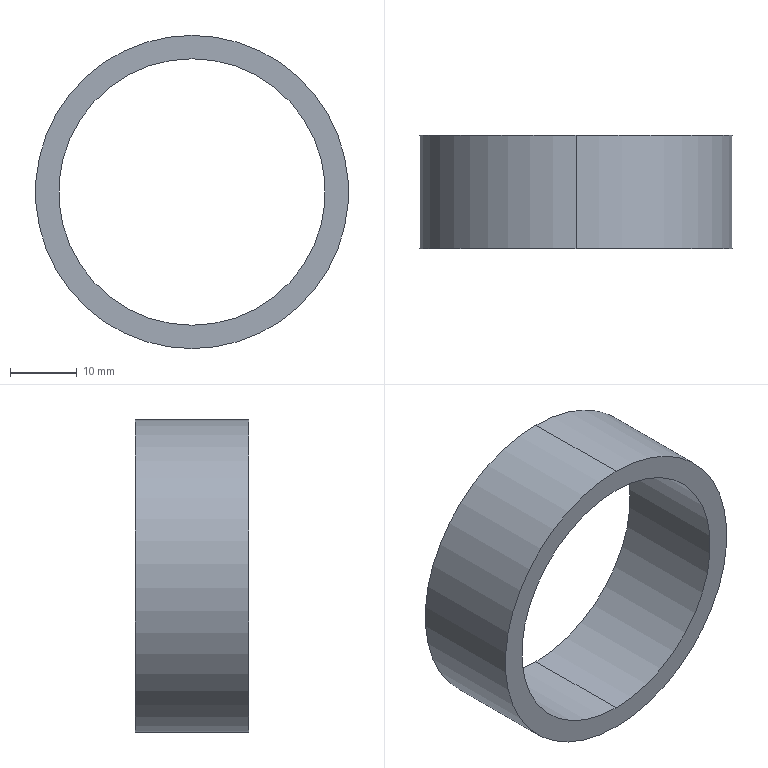Part | STEP file | 06-Spacer | 1 solid | 6 faces | box 47 x 17 x 47 mm | volume 8131 mm3 | cylinder 4 | plane 2 | commonest cylinder face diameters 40 x2 47 x2
STEP:
#1=CARTESIAN_POINT('',(0.,0.,0.));
#2=DIRECTION('',(0.,0.,1.));
#3=DIRECTION('',(1.,0.,0.));
#4=AXIS2_PLACEMENT_3D('',#1,#2,#3);
#5=CARTESIAN_POINT('',(0.,17.,-20.));
#6=VERTEX_POINT('',#5);
#7=CARTESIAN_POINT('',(0.,0.,-20.));
#8=VERTEX_POINT('',#7);
#9=CARTESIAN_POINT('',(0.,17.,-20.));
#10=DIRECTION('',(0.,-1.,0.));
#11=VECTOR('',#10,1.);
#12=LINE('',#9,#11);
#13=CARTESIAN_POINT('',(0.,17.,0.));
#14=DIRECTION('',(0.,-1.,0.));
#15=DIRECTION('',(0.,0.,-1.));
#16=AXIS2_PLACEMENT_3D('',#13,#14,#15);
#17=CYLINDRICAL_SURFACE('',#16,20.);
#18=CARTESIAN_POINT('',(6.283,0.));
#19=DIRECTION('',(0.,1.));
#20=VECTOR('',#19,1.);
#21=LINE('',#18,#20);
#22=(GEOMETRIC_REPRESENTATION_CONTEXT(2)PARAMETRIC_REPRESENTATION_CONTEXT()REPRESENTATION_CONTEXT('',''));
#23=DEFINITIONAL_REPRESENTATION('',(#21),#22);
#24=PCURVE('',#17,#23);
#25=CARTESIAN_POINT('',(0.,17.,0.));
#26=DIRECTION('',(0.,-1.,0.));
#27=DIRECTION('',(0.,0.,-1.));
#28=AXIS2_PLACEMENT_3D('',#25,#26,#27);
#29=CYLINDRICAL_SURFACE('',#28,20.);
#30=CARTESIAN_POINT('',(0.,0.));
#31=DIRECTION('',(0.,1.));
#32=VECTOR('',#31,1.);
#33=LINE('',#30,#32);
#34=(GEOMETRIC_REPRESENTATION_CONTEXT(2)PARAMETRIC_REPRESENTATION_CONTEXT()REPRESENTATION_CONTEXT('',''));
#35=DEFINITIONAL_REPRESENTATION('',(#33),#34);
#36=PCURVE('',#29,#35);
#37=SURFACE_CURVE('',#12,(#24,#36),.PCURVE_S1.);
#38=EDGE_CURVE('',#6,#8,#37,.T.);
#39=ORIENTED_EDGE('',*,*,#38,.T.);
#40=CARTESIAN_POINT('',(0.,0.,20.));
#41=VERTEX_POINT('',#40);
#42=CARTESIAN_POINT('',(0.,0.,0.));
#43=DIRECTION('',(0.,1.,0.));
#44=DIRECTION('',(0.,0.,1.));
#45=AXIS2_PLACEMENT_3D('',#42,#43,#44);
#46=CIRCLE('',#45,20.);
#47=CARTESIAN_POINT('',(9.425,17.));
#48=DIRECTION('',(-1.,0.));
#49=VECTOR('',#48,1.);
#50=LINE('',#47,#49);
#51=(GEOMETRIC_REPRESENTATION_CONTEXT(2)PARAMETRIC_REPRESENTATION_CONTEXT()REPRESENTATION_CONTEXT('',''));
#52=DEFINITIONAL_REPRESENTATION('',(#50),#51);
#53=PCURVE('',#17,#52);
#54=CARTESIAN_POINT('',(0.,0.,0.));
#55=DIRECTION('',(0.,1.,0.));
#56=DIRECTION('',(0.,0.,1.));
#57=AXIS2_PLACEMENT_3D('',#54,#55,#56);
#58=PLANE('',#57);
#59=CARTESIAN_POINT('',(0.,0.));
#60=DIRECTION('',(1.,0.));
#61=AXIS2_PLACEMENT_2D('',#59,#60);
#62=CIRCLE('',#61,20.);
#63=(GEOMETRIC_REPRESENTATION_CONTEXT(2)PARAMETRIC_REPRESENTATION_CONTEXT()REPRESENTATION_CONTEXT('',''));
#64=DEFINITIONAL_REPRESENTATION('',(#62),#63);
#65=PCURVE('',#58,#64);
#66=SURFACE_CURVE('',#46,(#53,#65),.PCURVE_S1.);
#67=EDGE_CURVE('',#8,#41,#66,.T.);
#68=ORIENTED_EDGE('',*,*,#67,.T.);
#69=CARTESIAN_POINT('',(0.,17.,20.));
#70=VERTEX_POINT('',#69);
#71=CARTESIAN_POINT('',(0.,17.,20.));
#72=DIRECTION('',(0.,-1.,0.));
#73=VECTOR('',#72,1.);
#74=LINE('',#71,#73);
#75=CARTESIAN_POINT('',(3.142,0.));
#76=DIRECTION('',(0.,1.));
#77=VECTOR('',#76,1.);
#78=LINE('',#75,#77);
#79=(GEOMETRIC_REPRESENTATION_CONTEXT(2)PARAMETRIC_REPRESENTATION_CONTEXT()REPRESENTATION_CONTEXT('',''));
#80=DEFINITIONAL_REPRESENTATION('',(#78),#79);
#81=PCURVE('',#17,#80);
#82=CARTESIAN_POINT('',(3.142,0.));
#83=DIRECTION('',(0.,1.));
#84=VECTOR('',#83,1.);
#85=LINE('',#82,#84);
#86=(GEOMETRIC_REPRESENTATION_CONTEXT(2)PARAMETRIC_REPRESENTATION_CONTEXT()REPRESENTATION_CONTEXT('',''));
#87=DEFINITIONAL_REPRESENTATION('',(#85),#86);
#88=PCURVE('',#29,#87);
#89=SURFACE_CURVE('',#74,(#81,#88),.PCURVE_S1.);
#90=EDGE_CURVE('',#70,#41,#89,.T.);
#91=ORIENTED_EDGE('',*,*,#90,.F.);
#92=CARTESIAN_POINT('',(0.,17.,0.));
#93=DIRECTION('',(0.,1.,0.));
#94=DIRECTION('',(0.,0.,1.));
#95=AXIS2_PLACEMENT_3D('',#92,#93,#94);
#96=CIRCLE('',#95,20.);
#97=CARTESIAN_POINT('',(9.425,0.));
#98=DIRECTION('',(-1.,0.));
#99=VECTOR('',#98,1.);
#100=LINE('',#97,#99);
#101=(GEOMETRIC_REPRESENTATION_CONTEXT(2)PARAMETRIC_REPRESENTATION_CONTEXT()REPRESENTATION_CONTEXT('',''));
#102=DEFINITIONAL_REPRESENTATION('',(#100),#101);
#103=PCURVE('',#17,#102);
#104=CARTESIAN_POINT('',(0.,17.,0.));
#105=DIRECTION('',(0.,1.,0.));
#106=DIRECTION('',(0.,0.,1.));
#107=AXIS2_PLACEMENT_3D('',#104,#105,#106);
#108=PLANE('',#107);
#109=CARTESIAN_POINT('',(0.,0.));
#110=DIRECTION('',(1.,0.));
#111=AXIS2_PLACEMENT_2D('',#109,#110);
#112=CIRCLE('',#111,20.);
#113=(GEOMETRIC_REPRESENTATION_CONTEXT(2)PARAMETRIC_REPRESENTATION_CONTEXT()REPRESENTATION_CONTEXT('',''));
#114=DEFINITIONAL_REPRESENTATION('',(#112),#113);
#115=PCURVE('',#108,#114);
#116=SURFACE_CURVE('',#96,(#103,#115),.PCURVE_S1.);
#117=EDGE_CURVE('',#6,#70,#116,.T.);
#118=ORIENTED_EDGE('',*,*,#117,.F.);
#119=EDGE_LOOP('',(#39,#68,#91,#118));
#120=FACE_BOUND('',#119,.F.);
#121=ADVANCED_FACE('',(#120),#17,.F.);
#122=CARTESIAN_POINT('',(0.,17.,23.5));
#123=VERTEX_POINT('',#122);
#124=CARTESIAN_POINT('',(0.,17.,-23.5));
#125=VERTEX_POINT('',#124);
#126=CARTESIAN_POINT('',(0.,17.,0.));
#127=DIRECTION('',(0.,1.,0.));
#128=DIRECTION('',(0.,0.,1.));
#129=AXIS2_PLACEMENT_3D('',#126,#127,#128);
#130=CIRCLE('',#129,23.5);
#131=CARTESIAN_POINT('',(0.,17.,0.));
#132=DIRECTION('',(0.,-1.,0.));
#133=DIRECTION('',(0.,0.,-1.));
#134=AXIS2_PLACEMENT_3D('',#131,#132,#133);
#135=CYLINDRICAL_SURFACE('',#134,23.5);
#136=CARTESIAN_POINT('',(3.142,0.));
#137=DIRECTION('',(-1.,0.));
#138=VECTOR('',#137,1.);
#139=LINE('',#136,#138);
#140=(GEOMETRIC_REPRESENTATION_CONTEXT(2)PARAMETRIC_REPRESENTATION_CONTEXT()REPRESENTATION_CONTEXT('',''));
#141=DEFINITIONAL_REPRESENTATION('',(#139),#140);
#142=PCURVE('',#135,#141);
#143=CARTESIAN_POINT('',(0.,0.));
#144=DIRECTION('',(1.,0.));
#145=AXIS2_PLACEMENT_2D('',#143,#144);
#146=CIRCLE('',#145,23.5);
#147=(GEOMETRIC_REPRESENTATION_CONTEXT(2)PARAMETRIC_REPRESENTATION_CONTEXT()REPRESENTATION_CONTEXT('',''));
#148=DEFINITIONAL_REPRESENTATION('',(#146),#147);
#149=PCURVE('',#108,#148);
#150=SURFACE_CURVE('',#130,(#142,#149),.PCURVE_S1.);
#151=EDGE_CURVE('',#123,#125,#150,.T.);
#152=ORIENTED_EDGE('',*,*,#151,.F.);
#153=CARTESIAN_POINT('',(0.,0.,23.5));
#154=VERTEX_POINT('',#153);
#155=CARTESIAN_POINT('',(0.,17.,23.5));
#156=DIRECTION('',(0.,-1.,0.));
#157=VECTOR('',#156,1.);
#158=LINE('',#155,#157);
#159=CARTESIAN_POINT('',(3.142,0.));
#160=DIRECTION('',(0.,1.));
#161=VECTOR('',#160,1.);
#162=LINE('',#159,#161);
#163=(GEOMETRIC_REPRESENTATION_CONTEXT(2)PARAMETRIC_REPRESENTATION_CONTEXT()REPRESENTATION_CONTEXT('',''));
#164=DEFINITIONAL_REPRESENTATION('',(#162),#163);
#165=PCURVE('',#135,#164);
#166=CARTESIAN_POINT('',(0.,17.,0.));
#167=DIRECTION('',(0.,-1.,0.));
#168=DIRECTION('',(0.,0.,-1.));
#169=AXIS2_PLACEMENT_3D('',#166,#167,#168);
#170=CYLINDRICAL_SURFACE('',#169,23.5);
#171=CARTESIAN_POINT('',(3.142,0.));
#172=DIRECTION('',(0.,1.));
#173=VECTOR('',#172,1.);
#174=LINE('',#171,#173);
#175=(GEOMETRIC_REPRESENTATION_CONTEXT(2)PARAMETRIC_REPRESENTATION_CONTEXT()REPRESENTATION_CONTEXT('',''));
#176=DEFINITIONAL_REPRESENTATION('',(#174),#175);
#177=PCURVE('',#170,#176);
#178=SURFACE_CURVE('',#158,(#165,#177),.PCURVE_S1.);
#179=EDGE_CURVE('',#123,#154,#178,.T.);
#180=ORIENTED_EDGE('',*,*,#179,.T.);
#181=CARTESIAN_POINT('',(0.,0.,-23.5));
#182=VERTEX_POINT('',#181);
#183=CARTESIAN_POINT('',(0.,0.,0.));
#184=DIRECTION('',(0.,1.,0.));
#185=DIRECTION('',(0.,0.,1.));
#186=AXIS2_PLACEMENT_3D('',#183,#184,#185);
#187=CIRCLE('',#186,23.5);
#188=CARTESIAN_POINT('',(3.142,17.));
#189=DIRECTION('',(-1.,0.));
#190=VECTOR('',#189,1.);
#191=LINE('',#188,#190);
#192=(GEOMETRIC_REPRESENTATION_CONTEXT(2)PARAMETRIC_REPRESENTATION_CONTEXT()REPRESENTATION_CONTEXT('',''));
#193=DEFINITIONAL_REPRESENTATION('',(#191),#192);
#194=PCURVE('',#135,#193);
#195=CARTESIAN_POINT('',(0.,0.));
#196=DIRECTION('',(1.,0.));
#197=AXIS2_PLACEMENT_2D('',#195,#196);
#198=CIRCLE('',#197,23.5);
#199=(GEOMETRIC_REPRESENTATION_CONTEXT(2)PARAMETRIC_REPRESENTATION_CONTEXT()REPRESENTATION_CONTEXT('',''));
#200=DEFINITIONAL_REPRESENTATION('',(#198),#199);
#201=PCURVE('',#58,#200);
#202=SURFACE_CURVE('',#187,(#194,#201),.PCURVE_S1.);
#203=EDGE_CURVE('',#154,#182,#202,.T.);
#204=ORIENTED_EDGE('',*,*,#203,.T.);
#205=CARTESIAN_POINT('',(0.,17.,-23.5));
#206=DIRECTION('',(0.,-1.,0.));
#207=VECTOR('',#206,1.);
#208=LINE('',#205,#207);
#209=CARTESIAN_POINT('',(0.,0.));
#210=DIRECTION('',(0.,1.));
#211=VECTOR('',#210,1.);
#212=LINE('',#209,#211);
#213=(GEOMETRIC_REPRESENTATION_CONTEXT(2)PARAMETRIC_REPRESENTATION_CONTEXT()REPRESENTATION_CONTEXT('',''));
#214=DEFINITIONAL_REPRESENTATION('',(#212),#213);
#215=PCURVE('',#135,#214);
#216=CARTESIAN_POINT('',(6.283,0.));
#217=DIRECTION('',(0.,1.));
#218=VECTOR('',#217,1.);
#219=LINE('',#216,#218);
#220=(GEOMETRIC_REPRESENTATION_CONTEXT(2)PARAMETRIC_REPRESENTATION_CONTEXT()REPRESENTATION_CONTEXT('',''));
#221=DEFINITIONAL_REPRESENTATION('',(#219),#220);
#222=PCURVE('',#170,#221);
#223=SURFACE_CURVE('',#208,(#215,#222),.PCURVE_S1.);
#224=EDGE_CURVE('',#125,#182,#223,.T.);
#225=ORIENTED_EDGE('',*,*,#224,.F.);
#226=EDGE_LOOP('',(#152,#180,#204,#225));
#227=FACE_BOUND('',#226,.T.);
#228=ADVANCED_FACE('',(#227),#135,.T.);
#229=CARTESIAN_POINT('',(0.,17.,0.));
#230=DIRECTION('',(0.,1.,0.));
#231=DIRECTION('',(0.,0.,1.));
#232=AXIS2_PLACEMENT_3D('',#229,#230,#231);
#233=CIRCLE('',#232,23.5);
#234=CARTESIAN_POINT('',(0.,0.));
#235=DIRECTION('',(1.,0.));
#236=AXIS2_PLACEMENT_2D('',#234,#235);
#237=CIRCLE('',#236,23.5);
#238=(GEOMETRIC_REPRESENTATION_CONTEXT(2)PARAMETRIC_REPRESENTATION_CONTEXT()REPRESENTATION_CONTEXT('',''));
#239=DEFINITIONAL_REPRESENTATION('',(#237),#238);
#240=PCURVE('',#108,#239);
#241=CARTESIAN_POINT('',(9.425,0.));
#242=DIRECTION('',(-1.,0.));
#243=VECTOR('',#242,1.);
#244=LINE('',#241,#243);
#245=(GEOMETRIC_REPRESENTATION_CONTEXT(2)PARAMETRIC_REPRESENTATION_CONTEXT()REPRESENTATION_CONTEXT('',''));
#246=DEFINITIONAL_REPRESENTATION('',(#244),#245);
#247=PCURVE('',#170,#246);
#248=SURFACE_CURVE('',#233,(#240,#247),.PCURVE_S1.);
#249=EDGE_CURVE('',#125,#123,#248,.T.);
#250=ORIENTED_EDGE('',*,*,#249,.T.);
#251=ORIENTED_EDGE('',*,*,#151,.T.);
#252=EDGE_LOOP('',(#250,#251));
#253=FACE_BOUND('',#252,.T.);
#254=ORIENTED_EDGE('',*,*,#117,.F.);
#255=CARTESIAN_POINT('',(0.,17.,0.));
#256=DIRECTION('',(0.,1.,0.));
#257=DIRECTION('',(0.,0.,1.));
#258=AXIS2_PLACEMENT_3D('',#255,#256,#257);
#259=CIRCLE('',#258,20.);
#260=CARTESIAN_POINT('',(0.,0.));
#261=DIRECTION('',(1.,0.));
#262=AXIS2_PLACEMENT_2D('',#260,#261);
#263=CIRCLE('',#262,20.);
#264=(GEOMETRIC_REPRESENTATION_CONTEXT(2)PARAMETRIC_REPRESENTATION_CONTEXT()REPRESENTATION_CONTEXT('',''));
#265=DEFINITIONAL_REPRESENTATION('',(#263),#264);
#266=PCURVE('',#108,#265);
#267=CARTESIAN_POINT('',(3.142,0.));
#268=DIRECTION('',(-1.,0.));
#269=VECTOR('',#268,1.);
#270=LINE('',#267,#269);
#271=(GEOMETRIC_REPRESENTATION_CONTEXT(2)PARAMETRIC_REPRESENTATION_CONTEXT()REPRESENTATION_CONTEXT('',''));
#272=DEFINITIONAL_REPRESENTATION('',(#270),#271);
#273=PCURVE('',#29,#272);
#274=SURFACE_CURVE('',#259,(#266,#273),.PCURVE_S1.);
#275=EDGE_CURVE('',#70,#6,#274,.T.);
#276=ORIENTED_EDGE('',*,*,#275,.F.);
#277=EDGE_LOOP('',(#254,#276));
#278=FACE_BOUND('',#277,.T.);
#279=ADVANCED_FACE('',(#253,#278),#108,.T.);
#280=CARTESIAN_POINT('',(0.,0.,0.));
#281=DIRECTION('',(0.,1.,0.));
#282=DIRECTION('',(0.,0.,1.));
#283=AXIS2_PLACEMENT_3D('',#280,#281,#282);
#284=CIRCLE('',#283,23.5);
#285=CARTESIAN_POINT('',(0.,0.));
#286=DIRECTION('',(1.,0.));
#287=AXIS2_PLACEMENT_2D('',#285,#286);
#288=CIRCLE('',#287,23.5);
#289=(GEOMETRIC_REPRESENTATION_CONTEXT(2)PARAMETRIC_REPRESENTATION_CONTEXT()REPRESENTATION_CONTEXT('',''));
#290=DEFINITIONAL_REPRESENTATION('',(#288),#289);
#291=PCURVE('',#58,#290);
#292=CARTESIAN_POINT('',(9.425,17.));
#293=DIRECTION('',(-1.,0.));
#294=VECTOR('',#293,1.);
#295=LINE('',#292,#294);
#296=(GEOMETRIC_REPRESENTATION_CONTEXT(2)PARAMETRIC_REPRESENTATION_CONTEXT()REPRESENTATION_CONTEXT('',''));
#297=DEFINITIONAL_REPRESENTATION('',(#295),#296);
#298=PCURVE('',#170,#297);
#299=SURFACE_CURVE('',#284,(#291,#298),.PCURVE_S1.);
#300=EDGE_CURVE('',#182,#154,#299,.T.);
#301=ORIENTED_EDGE('',*,*,#300,.F.);
#302=ORIENTED_EDGE('',*,*,#203,.F.);
#303=EDGE_LOOP('',(#301,#302));
#304=FACE_BOUND('',#303,.T.);
#305=ORIENTED_EDGE('',*,*,#67,.T.);
#306=CARTESIAN_POINT('',(0.,0.,0.));
#307=DIRECTION('',(0.,1.,0.));
#308=DIRECTION('',(0.,0.,1.));
#309=AXIS2_PLACEMENT_3D('',#306,#307,#308);
#310=CIRCLE('',#309,20.);
#311=CARTESIAN_POINT('',(0.,0.));
#312=DIRECTION('',(1.,0.));
#313=AXIS2_PLACEMENT_2D('',#311,#312);
#314=CIRCLE('',#313,20.);
#315=(GEOMETRIC_REPRESENTATION_CONTEXT(2)PARAMETRIC_REPRESENTATION_CONTEXT()REPRESENTATION_CONTEXT('',''));
#316=DEFINITIONAL_REPRESENTATION('',(#314),#315);
#317=PCURVE('',#58,#316);
#318=CARTESIAN_POINT('',(3.142,17.));
#319=DIRECTION('',(-1.,0.));
#320=VECTOR('',#319,1.);
#321=LINE('',#318,#320);
#322=(GEOMETRIC_REPRESENTATION_CONTEXT(2)PARAMETRIC_REPRESENTATION_CONTEXT()REPRESENTATION_CONTEXT('',''));
#323=DEFINITIONAL_REPRESENTATION('',(#321),#322);
#324=PCURVE('',#29,#323);
#325=SURFACE_CURVE('',#310,(#317,#324),.PCURVE_S1.);
#326=EDGE_CURVE('',#41,#8,#325,.T.);
#327=ORIENTED_EDGE('',*,*,#326,.T.);
#328=EDGE_LOOP('',(#305,#327));
#329=FACE_BOUND('',#328,.T.);
#330=ADVANCED_FACE('',(#304,#329),#58,.F.);
#331=ORIENTED_EDGE('',*,*,#179,.F.);
#332=ORIENTED_EDGE('',*,*,#249,.F.);
#333=ORIENTED_EDGE('',*,*,#224,.T.);
#334=ORIENTED_EDGE('',*,*,#300,.T.);
#335=EDGE_LOOP('',(#331,#332,#333,#334));
#336=FACE_BOUND('',#335,.T.);
#337=ADVANCED_FACE('',(#336),#170,.T.);
#338=ORIENTED_EDGE('',*,*,#326,.T.);
#339=ORIENTED_EDGE('',*,*,#38,.F.);
#340=ORIENTED_EDGE('',*,*,#275,.F.);
#341=ORIENTED_EDGE('',*,*,#90,.T.);
#342=EDGE_LOOP('',(#338,#339,#340,#341));
#343=FACE_BOUND('',#342,.F.);
#344=ADVANCED_FACE('',(#343),#29,.F.);
#345=CLOSED_SHELL('',(#121,#228,#279,#330,#337,#344));
#346=MANIFOLD_SOLID_BREP('',#345);
#347=(LENGTH_UNIT()NAMED_UNIT(*)SI_UNIT(.MILLI.,.METRE.));
#348=UNCERTAINTY_MEASURE_WITH_UNIT(LENGTH_MEASURE(0.0000001),#347,'','');
#349=(NAMED_UNIT(*)PLANE_ANGLE_UNIT()SI_UNIT($,.RADIAN.));
#350=(NAMED_UNIT(*)SI_UNIT($,.STERADIAN.)SOLID_ANGLE_UNIT());
#351=(GEOMETRIC_REPRESENTATION_CONTEXT(3)GLOBAL_UNCERTAINTY_ASSIGNED_CONTEXT((#348))GLOBAL_UNIT_ASSIGNED_CONTEXT((#347,#349,#350))REPRESENTATION_CONTEXT('',''));
#352=ADVANCED_BREP_SHAPE_REPRESENTATION('',(#4,#346),#351);